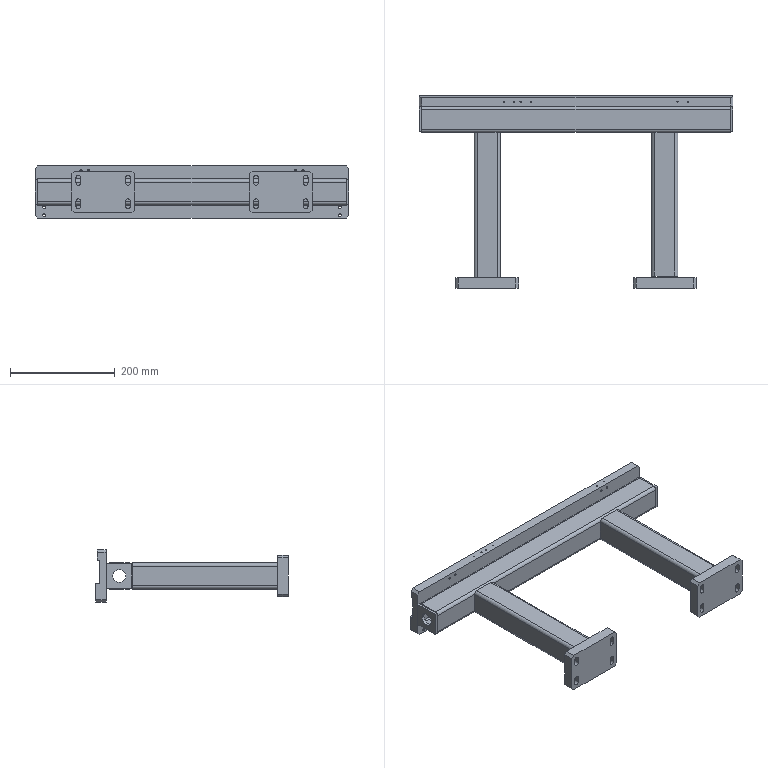Part | SolidWorks | features HoleWzd 1, MirrorStock 1 | 8 solids | 251 faces | box 600 x 368.308 x 100 mm | volume 1935248 mm3 | cylinder 110 | plane 92 | cone 49 | commonest cylinder face diameters 9 x24 3.3 x18 4.2 x16 6 x16 2.5 x12 12 x12